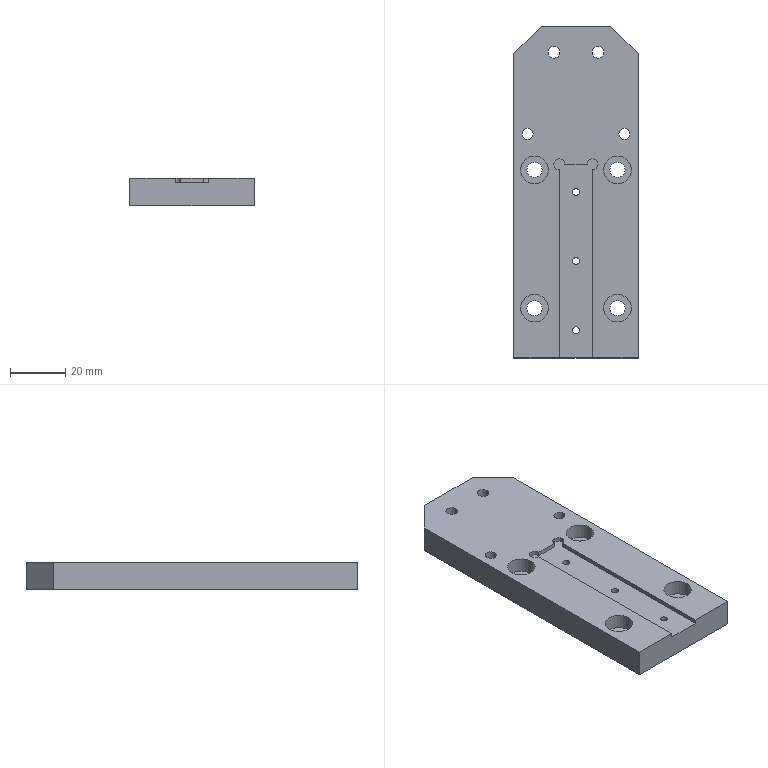Part | STEP file | E02 | 1 solid | 49 faces | box 45 x 120 x 10 mm | volume 48925 mm3 | cylinder 33 | plane 16 | commonest cylinder face diameters 5.5 x8 10 x8 4 x7 2.5 x6 4.2 x4